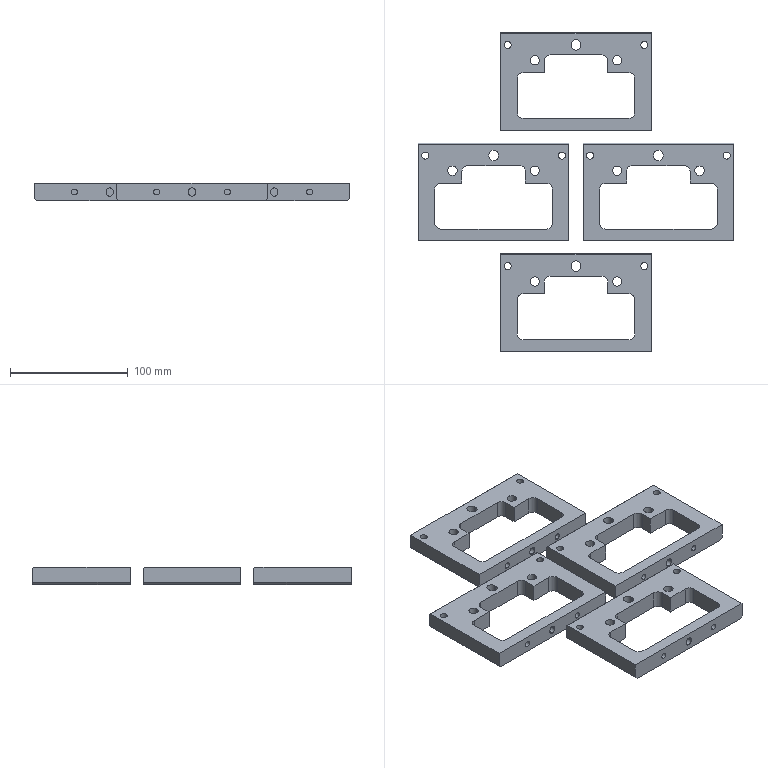NC program | NX | posted with a generic post | part box 268 x 271 x 15 mm
Lines 11494 to 12247 of 34527:
(HOLE_MILLING , TOOL : D4)
N22950 T04 M6
N22952 G54
N22954 G17 G0 G90 X-35. Y112. B0. C0. S9500 M3
N22956 G43 Z30. H4
N22958 Z0.5
N22960 G94 G3 X-34.05 Y111.05 R0.95 F1650.
N22962 X-33.1 Y112. R0.95
N22964 X-33.1 Y112. Z0.1 I-1.9 J0.
N22966 X-33.1 Y112. Z-0.3 I-1.9 J0.
N22968 X-33.1 Y112. Z-0.7 I-1.9 J0.
N22970 X-33.1 Y112. Z-1.1 I-1.9 J0.
N22972 X-33.1 Y112. Z-1.5 I-1.9 J0.
N22974 X-33.1 Y112. Z-1.9 I-1.9 J0.
N22976 X-33.1 Y112. Z-2.3 I-1.9 J0.
N22978 X-33.1 Y112. Z-2.7 I-1.9 J0.
N22980 X-33.1 Y112. Z-3.1 I-1.9 J0.
N22982 X-33.1 Y112. Z-3.5 I-1.9 J0.
N22984 X-33.1 Y112. Z-3.9 I-1.9 J0.
N22986 X-33.1 Y112. Z-4.3 I-1.9 J0.
N22988 X-33.1 Y112. Z-4.7 I-1.9 J0.
N22990 X-33.1 Y112. Z-5.1 I-1.9 J0.
N22992 X-33.1 Y112. Z-5.5 I-1.9 J0.
N22994 X-33.1 Y112. Z-5.9 I-1.9 J0.
N22996 X-33.1 Y112. Z-6.3 I-1.9 J0.
N22998 X-33.1 Y112. Z-6.7 I-1.9 J0.
N23000 X-33.1 Y112. Z-7.1 I-1.9 J0.
N23002 X-33.1 Y112. Z-7.5 I-1.9 J0.
N23004 X-33.1 Y112. Z-7.9 I-1.9 J0.
N23006 X-33.1 Y112. Z-8.3 I-1.9 J0.
N23008 X-33.1 Y112. Z-8.7 I-1.9 J0.
N23010 X-33.1 Y112. Z-9.1 I-1.9 J0.
N23012 X-33.1 Y112. Z-9.5 I-1.9 J0.
N23014 X-33.1 Y112. Z-9.9 I-1.9 J0.
N23016 X-33.1 Y112. Z-10.3 I-1.9 J0.
N23018 X-33.1 Y112. Z-10.7 I-1.9 J0.
N23020 X-33.1 Y112. Z-11.1 I-1.9 J0.
N23022 X-33.1 Y112. Z-11.5 I-1.9 J0.
N23024 X-33.1 Y112. Z-11.9 I-1.9 J0.
N23026 X-33.1 Y112. Z-12.3 I-1.9 J0.
N23028 X-33.1 Y112. Z-12.7 I-1.9 J0.
N23030 X-33.1 Y112. Z-13.1 I-1.9 J0.
N23032 X-33.1 Y112. Z-13.5 I-1.9 J0.
N23034 X-33.1 Y112. Z-13.9 I-1.9 J0.
N23036 X-33.1 Y112. Z-14.3 I-1.9 J0.
N23038 X-33.1 Y112. Z-14.7 I-1.9 J0.
N23040 X-35. Y110.1 Z-15. R-1.9
N23042 X-33.1 Y112. R1.9
N23044 X-35. Y110.1 R-1.9
N23046 X-34.05 Y111.05 R0.95
N23048 X-35. Y112. R0.95
N23050 G0 Z30.
N23052 X35.
N23054 Z0.5
N23056 G3 X35.95 Y111.05 R0.95
N23058 X36.9 Y112. R0.95
N23060 X36.9 Y112. Z0.1 I-1.9 J0.
N23062 X36.9 Y112. Z-0.3 I-1.9 J0.
N23064 X36.9 Y112. Z-0.7 I-1.9 J0.
N23066 X36.9 Y112. Z-1.1 I-1.9 J0.
N23068 X36.9 Y112. Z-1.5 I-1.9 J0.
N23070 X36.9 Y112. Z-1.9 I-1.9 J0.
N23072 X36.9 Y112. Z-2.3 I-1.9 J0.
N23074 X36.9 Y112. Z-2.7 I-1.9 J0.
N23076 X36.9 Y112. Z-3.1 I-1.9 J0.
N23078 X36.9 Y112. Z-3.5 I-1.9 J0.
N23080 X36.9 Y112. Z-3.9 I-1.9 J0.
N23082 X36.9 Y112. Z-4.3 I-1.9 J0.
N23084 X36.9 Y112. Z-4.7 I-1.9 J0.
N23086 X36.9 Y112. Z-5.1 I-1.9 J0.
N23088 X36.9 Y112. Z-5.5 I-1.9 J0.
N23090 X36.9 Y112. Z-5.9 I-1.9 J0.
N23092 X36.9 Y112. Z-6.3 I-1.9 J0.
N23094 X36.9 Y112. Z-6.7 I-1.9 J0.
N23096 X36.9 Y112. Z-7.1 I-1.9 J0.
N23098 X36.9 Y112. Z-7.5 I-1.9 J0.
N23100 X36.9 Y112. Z-7.9 I-1.9 J0.
N23102 X36.9 Y112. Z-8.3 I-1.9 J0.
N23104 X36.9 Y112. Z-8.7 I-1.9 J0.
N23106 X36.9 Y112. Z-9.1 I-1.9 J0.
N23108 X36.9 Y112. Z-9.5 I-1.9 J0.
N23110 X36.9 Y112. Z-9.9 I-1.9 J0.
N23112 X36.9 Y112. Z-10.3 I-1.9 J0.
N23114 X36.9 Y112. Z-10.7 I-1.9 J0.
N23116 X36.9 Y112. Z-11.1 I-1.9 J0.
N23118 X36.9 Y112. Z-11.5 I-1.9 J0.
N23120 X36.9 Y112. Z-11.9 I-1.9 J0.
N23122 X36.9 Y112. Z-12.3 I-1.9 J0.
N23124 X36.9 Y112. Z-12.7 I-1.9 J0.
N23126 X36.9 Y112. Z-13.1 I-1.9 J0.
N23128 X36.9 Y112. Z-13.5 I-1.9 J0.
N23130 X36.9 Y112. Z-13.9 I-1.9 J0.
N23132 X36.9 Y112. Z-14.3 I-1.9 J0.
N23134 X36.9 Y112. Z-14.7 I-1.9 J0.
N23136 X35. Y110.1 Z-15. R-1.9
N23138 X36.9 Y112. R1.9
N23140 X35. Y110.1 R-1.9
N23142 X35.95 Y111.05 R0.95
N23144 X35. Y112. R0.95
N23146 G0 Z30.
N23148 X105. Y18.
N23150 Z0.5
N23152 G3 X105.95 Y17.05 R0.95
N23154 X106.9 Y18. R0.95
N23156 X106.9 Y18. Z0.1 I-1.9 J0.
N23158 X106.9 Y18. Z-0.3 I-1.9 J0.
N23160 X106.9 Y18. Z-0.7 I-1.9 J0.
N23162 X106.9 Y18. Z-1.1 I-1.9 J0.
N23164 X106.9 Y18. Z-1.5 I-1.9 J0.
N23166 X106.9 Y18. Z-1.9 I-1.9 J0.
N23168 X106.9 Y18. Z-2.3 I-1.9 J0.
N23170 X106.9 Y18. Z-2.7 I-1.9 J0.
N23172 X106.9 Y18. Z-3.1 I-1.9 J0.
N23174 X106.9 Y18. Z-3.5 I-1.9 J0.
N23176 X106.9 Y18. Z-3.9 I-1.9 J0.
N23178 X106.9 Y18. Z-4.3 I-1.9 J0.
N23180 X106.9 Y18. Z-4.7 I-1.9 J0.
N23182 X106.9 Y18. Z-5.1 I-1.9 J0.
N23184 X106.9 Y18. Z-5.5 I-1.9 J0.
N23186 X106.9 Y18. Z-5.9 I-1.9 J0.
N23188 X106.9 Y18. Z-6.3 I-1.9 J0.
N23190 X106.9 Y18. Z-6.7 I-1.9 J0.
N23192 X106.9 Y18. Z-7.1 I-1.9 J0.
N23194 X106.9 Y18. Z-7.5 I-1.9 J0.
N23196 X106.9 Y18. Z-7.9 I-1.9 J0.
N23198 X106.9 Y18. Z-8.3 I-1.9 J0.
N23200 X106.9 Y18. Z-8.7 I-1.9 J0.
N23202 X106.9 Y18. Z-9.1 I-1.9 J0.
N23204 X106.9 Y18. Z-9.5 I-1.9 J0.
N23206 X106.9 Y18. Z-9.9 I-1.9 J0.
N23208 X106.9 Y18. Z-10.3 I-1.9 J0.
N23210 X106.9 Y18. Z-10.7 I-1.9 J0.
N23212 X106.9 Y18. Z-11.1 I-1.9 J0.
N23214 X106.9 Y18. Z-11.5 I-1.9 J0.
N23216 X106.9 Y18. Z-11.9 I-1.9 J0.
N23218 X106.9 Y18. Z-12.3 I-1.9 J0.
N23220 X106.9 Y18. Z-12.7 I-1.9 J0.
N23222 X106.9 Y18. Z-13.1 I-1.9 J0.
N23224 X106.9 Y18. Z-13.5 I-1.9 J0.
N23226 X106.9 Y18. Z-13.9 I-1.9 J0.
N23228 X106.9 Y18. Z-14.3 I-1.9 J0.
N23230 X106.9 Y18. Z-14.7 I-1.9 J0.
N23232 X105. Y16.1 Z-15. R-1.9
N23234 X106.9 Y18. R1.9
N23236 X105. Y16.1 R-1.9
N23238 X105.95 Y17.05 R0.95
N23240 X105. Y18. R0.95
N23242 G0 Z30.
N23244 X35.
N23246 Z0.5
N23248 G3 X35.95 Y17.05 R0.95
N23250 X36.9 Y18. R0.95
N23252 X36.9 Y18. Z0.1 I-1.9 J0.
N23254 X36.9 Y18. Z-0.3 I-1.9 J0.
N23256 X36.9 Y18. Z-0.7 I-1.9 J0.
N23258 X36.9 Y18. Z-1.1 I-1.9 J0.
N23260 X36.9 Y18. Z-1.5 I-1.9 J0.
N23262 X36.9 Y18. Z-1.9 I-1.9 J0.
N23264 X36.9 Y18. Z-2.3 I-1.9 J0.
N23266 X36.9 Y18. Z-2.7 I-1.9 J0.
N23268 X36.9 Y18. Z-3.1 I-1.9 J0.
N23270 X36.9 Y18. Z-3.5 I-1.9 J0.
N23272 X36.9 Y18. Z-3.9 I-1.9 J0.
N23274 X36.9 Y18. Z-4.3 I-1.9 J0.
N23276 X36.9 Y18. Z-4.7 I-1.9 J0.
N23278 X36.9 Y18. Z-5.1 I-1.9 J0.
N23280 X36.9 Y18. Z-5.5 I-1.9 J0.
N23282 X36.9 Y18. Z-5.9 I-1.9 J0.
N23284 X36.9 Y18. Z-6.3 I-1.9 J0.
N23286 X36.9 Y18. Z-6.7 I-1.9 J0.
N23288 X36.9 Y18. Z-7.1 I-1.9 J0.
N23290 X36.9 Y18. Z-7.5 I-1.9 J0.
N23292 X36.9 Y18. Z-7.9 I-1.9 J0.
N23294 X36.9 Y18. Z-8.3 I-1.9 J0.
N23296 X36.9 Y18. Z-8.7 I-1.9 J0.
N23298 X36.9 Y18. Z-9.1 I-1.9 J0.
N23300 X36.9 Y18. Z-9.5 I-1.9 J0.
N23302 X36.9 Y18. Z-9.9 I-1.9 J0.
N23304 X36.9 Y18. Z-10.3 I-1.9 J0.
N23306 X36.9 Y18. Z-10.7 I-1.9 J0.
N23308 X36.9 Y18. Z-11.1 I-1.9 J0.
N23310 X36.9 Y18. Z-11.5 I-1.9 J0.
N23312 X36.9 Y18. Z-11.9 I-1.9 J0.
N23314 X36.9 Y18. Z-12.3 I-1.9 J0.
N23316 X36.9 Y18. Z-12.7 I-1.9 J0.
N23318 X36.9 Y18. Z-13.1 I-1.9 J0.
N23320 X36.9 Y18. Z-13.5 I-1.9 J0.
N23322 X36.9 Y18. Z-13.9 I-1.9 J0.
N23324 X36.9 Y18. Z-14.3 I-1.9 J0.
N23326 X36.9 Y18. Z-14.7 I-1.9 J0.
N23328 X35. Y16.1 Z-15. R-1.9
N23330 X36.9 Y18. R1.9
N23332 X35. Y16.1 R-1.9
N23334 X35.95 Y17.05 R0.95
N23336 X35. Y18. R0.95
N23338 G0 Z30.
N23340 Y-76.
N23342 Z0.5
N23344 G3 X35.95 Y-76.95 R0.95
N23346 X36.9 Y-76. R0.95
N23348 X36.9 Y-76. Z0.1 I-1.9 J0.
N23350 X36.9 Y-76. Z-0.3 I-1.9 J0.
N23352 X36.9 Y-76. Z-0.7 I-1.9 J0.
N23354 X36.9 Y-76. Z-1.1 I-1.9 J0.
N23356 X36.9 Y-76. Z-1.5 I-1.9 J0.
N23358 X36.9 Y-76. Z-1.9 I-1.9 J0.
N23360 X36.9 Y-76. Z-2.3 I-1.9 J0.
N23362 X36.9 Y-76. Z-2.7 I-1.9 J0.
N23364 X36.9 Y-76. Z-3.1 I-1.9 J0.
N23366 X36.9 Y-76. Z-3.5 I-1.9 J0.
N23368 X36.9 Y-76. Z-3.9 I-1.9 J0.
N23370 X36.9 Y-76. Z-4.3 I-1.9 J0.
N23372 X36.9 Y-76. Z-4.7 I-1.9 J0.
N23374 X36.9 Y-76. Z-5.1 I-1.9 J0.
N23376 X36.9 Y-76. Z-5.5 I-1.9 J0.
N23378 X36.9 Y-76. Z-5.9 I-1.9 J0.
N23380 X36.9 Y-76. Z-6.3 I-1.9 J0.
N23382 X36.9 Y-76. Z-6.7 I-1.9 J0.
N23384 X36.9 Y-76. Z-7.1 I-1.9 J0.
N23386 X36.9 Y-76. Z-7.5 I-1.9 J0.
N23388 X36.9 Y-76. Z-7.9 I-1.9 J0.
N23390 X36.9 Y-76. Z-8.3 I-1.9 J0.
N23392 X36.9 Y-76. Z-8.7 I-1.9 J0.
N23394 X36.9 Y-76. Z-9.1 I-1.9 J0.
N23396 X36.9 Y-76. Z-9.5 I-1.9 J0.
N23398 X36.9 Y-76. Z-9.9 I-1.9 J0.
N23400 X36.9 Y-76. Z-10.3 I-1.9 J0.
N23402 X36.9 Y-76. Z-10.7 I-1.9 J0.
N23404 X36.9 Y-76. Z-11.1 I-1.9 J0.
N23406 X36.9 Y-76. Z-11.5 I-1.9 J0.
N23408 X36.9 Y-76. Z-11.9 I-1.9 J0.
N23410 X36.9 Y-76. Z-12.3 I-1.9 J0.
N23412 X36.9 Y-76. Z-12.7 I-1.9 J0.
N23414 X36.9 Y-76. Z-13.1 I-1.9 J0.
N23416 X36.9 Y-76. Z-13.5 I-1.9 J0.
N23418 X36.9 Y-76. Z-13.9 I-1.9 J0.
N23420 X36.9 Y-76. Z-14.3 I-1.9 J0.
N23422 X36.9 Y-76. Z-14.7 I-1.9 J0.
N23424 X35. Y-77.9 Z-15. R-1.9
N23426 X36.9 Y-76. R1.9
N23428 X35. Y-77.9 R-1.9
N23430 X35.95 Y-76.95 R0.95
N23432 X35. Y-76. R0.95
N23434 G0 Z30.
N23436 X-35.
N23438 Z0.5
N23440 G3 X-34.05 Y-76.95 R0.95
N23442 X-33.1 Y-76. R0.95
N23444 X-33.1 Y-76. Z0.1 I-1.9 J0.
N23446 X-33.1 Y-76. Z-0.3 I-1.9 J0.
N23448 X-33.1 Y-76. Z-0.7 I-1.9 J0.
N23450 X-33.1 Y-76. Z-1.1 I-1.9 J0.
N23452 X-33.1 Y-76. Z-1.5 I-1.9 J0.
N23454 X-33.1 Y-76. Z-1.9 I-1.9 J0.
N23456 X-33.1 Y-76. Z-2.3 I-1.9 J0.
N23458 X-33.1 Y-76. Z-2.7 I-1.9 J0.
N23460 X-33.1 Y-76. Z-3.1 I-1.9 J0.
N23462 X-33.1 Y-76. Z-3.5 I-1.9 J0.
N23464 X-33.1 Y-76. Z-3.9 I-1.9 J0.
N23466 X-33.1 Y-76. Z-4.3 I-1.9 J0.
N23468 X-33.1 Y-76. Z-4.7 I-1.9 J0.
N23470 X-33.1 Y-76. Z-5.1 I-1.9 J0.
N23472 X-33.1 Y-76. Z-5.5 I-1.9 J0.
N23474 X-33.1 Y-76. Z-5.9 I-1.9 J0.
N23476 X-33.1 Y-76. Z-6.3 I-1.9 J0.
N23478 X-33.1 Y-76. Z-6.7 I-1.9 J0.
N23480 X-33.1 Y-76. Z-7.1 I-1.9 J0.
N23482 X-33.1 Y-76. Z-7.5 I-1.9 J0.
N23484 X-33.1 Y-76. Z-7.9 I-1.9 J0.
N23486 X-33.1 Y-76. Z-8.3 I-1.9 J0.
N23488 X-33.1 Y-76. Z-8.7 I-1.9 J0.
N23490 X-33.1 Y-76. Z-9.1 I-1.9 J0.
N23492 X-33.1 Y-76. Z-9.5 I-1.9 J0.
N23494 X-33.1 Y-76. Z-9.9 I-1.9 J0.
N23496 X-33.1 Y-76. Z-10.3 I-1.9 J0.
N23498 X-33.1 Y-76. Z-10.7 I-1.9 J0.
N23500 X-33.1 Y-76. Z-11.1 I-1.9 J0.
N23502 X-33.1 Y-76. Z-11.5 I-1.9 J0.
N23504 X-33.1 Y-76. Z-11.9 I-1.9 J0.
N23506 X-33.1 Y-76. Z-12.3 I-1.9 J0.
N23508 X-33.1 Y-76. Z-12.7 I-1.9 J0.
N23510 X-33.1 Y-76. Z-13.1 I-1.9 J0.
N23512 X-33.1 Y-76. Z-13.5 I-1.9 J0.
N23514 X-33.1 Y-76. Z-13.9 I-1.9 J0.
N23516 X-33.1 Y-76. Z-14.3 I-1.9 J0.
N23518 X-33.1 Y-76. Z-14.7 I-1.9 J0.
N23520 X-35. Y-77.9 Z-15. R-1.9
N23522 X-33.1 Y-76. R1.9
N23524 X-35. Y-77.9 R-1.9
N23526 X-34.05 Y-76.95 R0.95
N23528 X-35. Y-76. R0.95
N23530 G0 Z30.
N23532 Y18.
N23534 Z0.5
N23536 G3 X-34.05 Y17.05 R0.95
N23538 X-33.1 Y18. R0.95
N23540 X-33.1 Y18. Z0.1 I-1.9 J0.
N23542 X-33.1 Y18. Z-0.3 I-1.9 J0.
N23544 X-33.1 Y18. Z-0.7 I-1.9 J0.
N23546 X-33.1 Y18. Z-1.1 I-1.9 J0.
N23548 X-33.1 Y18. Z-1.5 I-1.9 J0.
N23550 X-33.1 Y18. Z-1.9 I-1.9 J0.
N23552 X-33.1 Y18. Z-2.3 I-1.9 J0.
N23554 X-33.1 Y18. Z-2.7 I-1.9 J0.
N23556 X-33.1 Y18. Z-3.1 I-1.9 J0.
N23558 X-33.1 Y18. Z-3.5 I-1.9 J0.
N23560 X-33.1 Y18. Z-3.9 I-1.9 J0.
N23562 X-33.1 Y18. Z-4.3 I-1.9 J0.
N23564 X-33.1 Y18. Z-4.7 I-1.9 J0.
N23566 X-33.1 Y18. Z-5.1 I-1.9 J0.
N23568 X-33.1 Y18. Z-5.5 I-1.9 J0.
N23570 X-33.1 Y18. Z-5.9 I-1.9 J0.
N23572 X-33.1 Y18. Z-6.3 I-1.9 J0.
N23574 X-33.1 Y18. Z-6.7 I-1.9 J0.
N23576 X-33.1 Y18. Z-7.1 I-1.9 J0.
N23578 X-33.1 Y18. Z-7.5 I-1.9 J0.
N23580 X-33.1 Y18. Z-7.9 I-1.9 J0.
N23582 X-33.1 Y18. Z-8.3 I-1.9 J0.
N23584 X-33.1 Y18. Z-8.7 I-1.9 J0.
N23586 X-33.1 Y18. Z-9.1 I-1.9 J0.
N23588 X-33.1 Y18. Z-9.5 I-1.9 J0.
N23590 X-33.1 Y18. Z-9.9 I-1.9 J0.
N23592 X-33.1 Y18. Z-10.3 I-1.9 J0.
N23594 X-33.1 Y18. Z-10.7 I-1.9 J0.
N23596 X-33.1 Y18. Z-11.1 I-1.9 J0.
N23598 X-33.1 Y18. Z-11.5 I-1.9 J0.
N23600 X-33.1 Y18. Z-11.9 I-1.9 J0.
N23602 X-33.1 Y18. Z-12.3 I-1.9 J0.
N23604 X-33.1 Y18. Z-12.7 I-1.9 J0.
N23606 X-33.1 Y18. Z-13.1 I-1.9 J0.
N23608 X-33.1 Y18. Z-13.5 I-1.9 J0.
N23610 X-33.1 Y18. Z-13.9 I-1.9 J0.
N23612 X-33.1 Y18. Z-14.3 I-1.9 J0.
N23614 X-33.1 Y18. Z-14.7 I-1.9 J0.
N23616 X-35. Y16.1 Z-15. R-1.9
N23618 X-33.1 Y18. R1.9
N23620 X-35. Y16.1 R-1.9
N23622 X-34.05 Y17.05 R0.95
N23624 X-35. Y18. R0.95
N23626 G0 Z30.
N23628 X-105.
N23630 Z0.5
N23632 G3 X-104.05 Y17.05 R0.95
N23634 X-103.1 Y18. R0.95
N23636 X-103.1 Y18. Z0.1 I-1.9 J0.
N23638 X-103.1 Y18. Z-0.3 I-1.9 J0.
N23640 X-103.1 Y18. Z-0.7 I-1.9 J0.
N23642 X-103.1 Y18. Z-1.1 I-1.9 J0.
N23644 X-103.1 Y18. Z-1.5 I-1.9 J0.
N23646 X-103.1 Y18. Z-1.9 I-1.9 J0.
N23648 X-103.1 Y18. Z-2.3 I-1.9 J0.
N23650 X-103.1 Y18. Z-2.7 I-1.9 J0.
N23652 X-103.1 Y18. Z-3.1 I-1.9 J0.
N23654 X-103.1 Y18. Z-3.5 I-1.9 J0.
N23656 X-103.1 Y18. Z-3.9 I-1.9 J0.
N23658 X-103.1 Y18. Z-4.3 I-1.9 J0.
N23660 X-103.1 Y18. Z-4.7 I-1.9 J0.
N23662 X-103.1 Y18. Z-5.1 I-1.9 J0.
N23664 X-103.1 Y18. Z-5.5 I-1.9 J0.
N23666 X-103.1 Y18. Z-5.9 I-1.9 J0.
N23668 X-103.1 Y18. Z-6.3 I-1.9 J0.
N23670 X-103.1 Y18. Z-6.7 I-1.9 J0.
N23672 X-103.1 Y18. Z-7.1 I-1.9 J0.
N23674 X-103.1 Y18. Z-7.5 I-1.9 J0.
N23676 X-103.1 Y18. Z-7.9 I-1.9 J0.
N23678 X-103.1 Y18. Z-8.3 I-1.9 J0.
N23680 X-103.1 Y18. Z-8.7 I-1.9 J0.
N23682 X-103.1 Y18. Z-9.1 I-1.9 J0.
N23684 X-103.1 Y18. Z-9.5 I-1.9 J0.
N23686 X-103.1 Y18. Z-9.9 I-1.9 J0.
N23688 X-103.1 Y18. Z-10.3 I-1.9 J0.
N23690 X-103.1 Y18. Z-10.7 I-1.9 J0.
N23692 X-103.1 Y18. Z-11.1 I-1.9 J0.
N23694 X-103.1 Y18. Z-11.5 I-1.9 J0.
N23696 X-103.1 Y18. Z-11.9 I-1.9 J0.
N23698 X-103.1 Y18. Z-12.3 I-1.9 J0.
N23700 X-103.1 Y18. Z-12.7 I-1.9 J0.
N23702 X-103.1 Y18. Z-13.1 I-1.9 J0.
N23704 X-103.1 Y18. Z-13.5 I-1.9 J0.
N23706 X-103.1 Y18. Z-13.9 I-1.9 J0.
N23708 X-103.1 Y18. Z-14.3 I-1.9 J0.
N23710 X-103.1 Y18. Z-14.7 I-1.9 J0.
N23712 X-105. Y16.1 Z-15. R-1.9
N23714 X-103.1 Y18. R1.9
N23716 X-105. Y16.1 R-1.9
N23718 X-104.05 Y17.05 R0.95
N23720 X-105. Y18. R0.95
N23722 G0 Z30.
(ZLEVEL_PROFILE_COPY , TOOL : D4)
N23724 X-68.65 Y32.83
N23726 Z1.5
N23728 G1 X-68.775 Y32.965 Z1.49 F1000.
N23730 X-69.188 Y33.229 Z1.465
N23732 X-69.557 Y33.358 Z1.444
N23734 X-70.095 Y33.408 Z1.416
N23736 X-70.625 Y33.305 Z1.388
N23738 X-71.105 Y33.058 Z1.359
N23740 X-71.497 Y32.686 Z1.331
N23742 X-71.769 Y32.219 Z1.303
N23744 X-71.9 Y31.695 Z1.274
N23746 Y30.305 Z1.201
N23748 X-71.785 Y29.822 Z1.175
N23750 X-71.61 Y29.473 Z1.155
N23752 X-71.289 Y29.091 Z1.129
N23754 X-70.881 Y28.805 Z1.103
N23756 X-70.412 Y28.635 Z1.077
N23758 X-69.915 Y28.592 Z1.05
N23760 X-69.424 Y28.679 Z1.024
N23762 X-68.973 Y28.89 Z0.998
N23764 X-68.591 Y29.211 Z0.972
N23766 X-68.358 Y29.524 Z0.952
N23768 X-68.187 Y29.9 Z0.93
N23770 X-68.1 Y30.305 Z0.908
N23772 Y31.695 Z0.835
N23774 X-68.212 Y32.172 Z0.81
N23776 X-68.442 Y32.605 Z0.784
N23778 X-68.775 Y32.965 Z0.758
N23780 X-69.188 Y33.229 Z0.733
N23782 X-69.557 Y33.358 Z0.712
N23784 X-70.095 Y33.408 Z0.684
N23786 X-70.625 Y33.305 Z0.656
N23788 X-71.105 Y33.058 Z0.627
N23790 X-71.497 Y32.686 Z0.599
N23792 X-71.769 Y32.219 Z0.571
N23794 X-71.9 Y31.695 Z0.542
N23796 Y30.305 Z0.469
N23798 X-71.785 Y29.822 Z0.443
N23800 X-71.61 Y29.473 Z0.423
N23802 X-71.289 Y29.091 Z0.397
N23804 X-70.881 Y28.805 Z0.371
N23806 X-70.412 Y28.635 Z0.345
N23808 X-69.915 Y28.592 Z0.318
N23810 X-69.424 Y28.679 Z0.292
N23812 X-68.973 Y28.89 Z0.266
N23814 X-68.591 Y29.211 Z0.24
N23816 X-68.358 Y29.524 Z0.22
N23818 X-68.187 Y29.9 Z0.198
N23820 X-68.1 Y30.305 Z0.176
N23822 Y31.695 Z0.103
N23824 X-68.212 Y32.172 Z0.078
N23826 X-68.442 Y32.605 Z0.052
N23828 X-68.775 Y32.965 Z0.026
N23830 X-69.188 Y33.229 Z0.001
N23832 X-69.557 Y33.358 Z-0.02
N23834 X-70.095 Y33.408 Z-0.048
N23836 X-70.625 Y33.305 Z-0.077
N23838 X-71.105 Y33.058 Z-0.105
N23840 X-71.497 Y32.686 Z-0.133
N23842 X-71.769 Y32.219 Z-0.161
N23844 X-71.9 Y31.695 Z-0.19
N23846 Y31.5 Z-0.2
N23848 Y30.5 F1200.
N23850 G3 X-70. Y28.6 R1.9
N23852 X-68.1 Y30.5 R1.9
N23854 G1 Y31.5
N23856 G3 X-70. Y33.4 R1.9
N23858 X-71.9 Y31.5 R1.9
N23860 G1 Y30.652 Z-0.216
N23862 X-71.897 Y30.511 Z-0.219
N23864 X-71.888 Y30.371 Z-0.222
N23866 X-71.877 Y30.23 Z-0.224
N23868 X-71.848 Y30.092 Z-0.227
N23870 X-71.814 Y29.956 Z-0.23
N23872 X-71.768 Y29.823 Z-0.232
N23874 X-71.713 Y29.693 Z-0.235
N23876 X-71.648 Y29.568 Z-0.238
N23878 X-71.574 Y29.449 Z-0.241
N23880 X-71.493 Y29.334 Z-0.243
N23882 X-71.401 Y29.227 Z-0.246
N23884 X-71.304 Y29.125 Z-0.249
N23886 X-71.197 Y29.034 Z-0.251
N23888 X-71.087 Y28.946 Z-0.254
N23890 X-70.966 Y28.873 Z-0.257
N23892 X-70.843 Y28.804 Z-0.259
N23894 X-70.714 Y28.747 Z-0.262
N23896 X-70.582 Y28.699 Z-0.265
N23898 X-70.447 Y28.66 Z-0.268
N23900 X-70.309 Y28.632 Z-0.27
N23902 X-70.17 Y28.614 Z-0.273
N23904 X-70.029 Y28.608 Z-0.276
N23906 X-69.888 Y28.609 Z-0.278
N23908 X-69.748 Y28.625 Z-0.281
N23910 X-69.609 Y28.645 Z-0.284
N23912 X-69.473 Y28.683 Z-0.286
N23914 X-69.339 Y28.724 Z-0.289
N23916 X-69.21 Y28.781 Z-0.292
N23918 X-69.083 Y28.843 Z-0.295
N23920 X-68.963 Y28.916 Z-0.297
N23922 X-68.849 Y28.998 Z-0.3
N23924 X-68.739 Y29.086 Z-0.303
N23926 X-68.634 Y29.18 Z-0.305
N23928 X-68.539 Y29.285 Z-0.308
N23930 X-68.453 Y29.397 Z-0.311
N23932 X-68.375 Y29.515 Z-0.314
N23934 X-68.307 Y29.638 Z-0.316
N23936 X-68.247 Y29.766 Z-0.319
N23938 X-68.198 Y29.898 Z-0.322
N23940 X-68.158 Y30.034 Z-0.324
N23942 X-68.129 Y30.172 Z-0.327
N23944 X-68.116 Y30.313 Z-0.33
N23946 X-68.106 Y30.453 Z-0.332
N23948 X-68.1 Y30.594 Z-0.335
N23950 Y31.442 Z-0.351
N23952 X-68.109 Y31.582 Z-0.354
N23954 X-68.119 Y31.723 Z-0.357
N23956 X-68.142 Y31.862 Z-0.359
N23958 X-68.172 Y32. Z-0.362
N23960 X-68.217 Y32.133 Z-0.365
N23962 X-68.266 Y32.265 Z-0.368
N23964 X-68.33 Y32.39 Z-0.37
N23966 X-68.399 Y32.513 Z-0.373
N23968 X-68.48 Y32.628 Z-0.376
N23970 X-68.568 Y32.738 Z-0.378
N23972 X-68.664 Y32.841 Z-0.381
N23974 X-68.767 Y32.937 Z-0.384
N23976 X-68.877 Y33.025 Z-0.386
N23978 X-68.994 Y33.102 Z-0.389
N23980 X-69.114 Y33.176 Z-0.392
N23982 X-69.243 Y33.234 Z-0.395
N23984 X-69.372 Y33.289 Z-0.397
N23986 X-69.506 Y33.335 Z-0.4
N23988 G3 X-71.9 Y31.5 R1.9
N23990 G1 Y30.652 Z-0.416
N23992 X-71.897 Y30.511 Z-0.419
N23994 X-71.888 Y30.371 Z-0.422
N23996 X-71.877 Y30.23 Z-0.424
N23998 X-71.848 Y30.092 Z-0.427
N24000 X-71.814 Y29.956 Z-0.43
N24002 X-71.768 Y29.823 Z-0.432
N24004 X-71.713 Y29.693 Z-0.435
N24006 X-71.648 Y29.568 Z-0.438
N24008 X-71.574 Y29.449 Z-0.441
N24010 X-71.493 Y29.334 Z-0.443
N24012 X-71.401 Y29.227 Z-0.446
N24014 X-71.304 Y29.125 Z-0.449
N24016 X-71.197 Y29.034 Z-0.451
N24018 X-71.087 Y28.946 Z-0.454
N24020 X-70.966 Y28.873 Z-0.457
N24022 X-70.843 Y28.804 Z-0.459
N24024 X-70.714 Y28.747 Z-0.462
N24026 X-70.582 Y28.699 Z-0.465
N24028 X-70.447 Y28.66 Z-0.468
N24030 X-70.309 Y28.632 Z-0.47
N24032 X-70.17 Y28.614 Z-0.473
N24034 X-70.029 Y28.608 Z-0.476
N24036 X-69.888 Y28.609 Z-0.478
N24038 X-69.748 Y28.625 Z-0.481
N24040 X-69.609 Y28.645 Z-0.484
N24042 X-69.473 Y28.683 Z-0.486
N24044 X-69.339 Y28.724 Z-0.489
N24046 X-69.21 Y28.781 Z-0.492
N24048 X-69.083 Y28.843 Z-0.495
N24050 X-68.963 Y28.916 Z-0.497
N24052 X-68.849 Y28.998 Z-0.5
N24054 X-68.739 Y29.086 Z-0.503
N24056 X-68.634 Y29.18 Z-0.505
N24058 X-68.539 Y29.285 Z-0.508
N24060 X-68.453 Y29.397 Z-0.511
N24062 X-68.375 Y29.515 Z-0.514
N24064 X-68.307 Y29.638 Z-0.516
N24066 X-68.247 Y29.766 Z-0.519
N24068 X-68.198 Y29.898 Z-0.522
N24070 X-68.158 Y30.034 Z-0.524
N24072 X-68.129 Y30.172 Z-0.527
N24074 X-68.116 Y30.313 Z-0.53
N24076 X-68.106 Y30.453 Z-0.532
N24078 X-68.1 Y30.594 Z-0.535
N24080 Y31.442 Z-0.551
N24082 X-68.109 Y31.582 Z-0.554
N24084 X-68.119 Y31.723 Z-0.557
N24086 X-68.142 Y31.862 Z-0.559
N24088 X-68.172 Y32. Z-0.562
N24090 X-68.217 Y32.133 Z-0.565
N24092 X-68.266 Y32.265 Z-0.568
N24094 X-68.33 Y32.39 Z-0.57
N24096 X-68.399 Y32.513 Z-0.573
N24098 X-68.48 Y32.628 Z-0.576
N24100 X-68.568 Y32.738 Z-0.578
N24102 X-68.664 Y32.841 Z-0.581
N24104 X-68.767 Y32.937 Z-0.584
N24106 X-68.877 Y33.025 Z-0.586
N24108 X-68.994 Y33.102 Z-0.589
N24110 X-69.114 Y33.176 Z-0.592
N24112 X-69.243 Y33.234 Z-0.595
N24114 X-69.372 Y33.289 Z-0.597
N24116 X-69.506 Y33.335 Z-0.6
N24118 G3 X-71.9 Y31.5 R1.9
N24120 G1 Y30.652 Z-0.616
N24122 X-71.897 Y30.511 Z-0.619
N24124 X-71.888 Y30.371 Z-0.622
N24126 X-71.877 Y30.23 Z-0.624
N24128 X-71.848 Y30.092 Z-0.627
N24130 X-71.814 Y29.956 Z-0.63
N24132 X-71.768 Y29.823 Z-0.632
N24134 X-71.713 Y29.693 Z-0.635
N24136 X-71.648 Y29.568 Z-0.638
N24138 X-71.574 Y29.449 Z-0.641
N24140 X-71.493 Y29.334 Z-0.643
N24142 X-71.401 Y29.227 Z-0.646
N24144 X-71.304 Y29.125 Z-0.649
N24146 X-71.197 Y29.034 Z-0.651
N24148 X-71.087 Y28.946 Z-0.654
N24150 X-70.966 Y28.873 Z-0.657
N24152 X-70.843 Y28.804 Z-0.659
N24154 X-70.714 Y28.747 Z-0.662
N24156 X-70.582 Y28.699 Z-0.665
N24158 X-70.447 Y28.66 Z-0.668
N24160 X-70.309 Y28.632 Z-0.67
N24162 X-70.17 Y28.614 Z-0.673
N24164 X-70.029 Y28.608 Z-0.676
N24166 X-69.888 Y28.609 Z-0.678
N24168 X-69.748 Y28.625 Z-0.681
N24170 X-69.609 Y28.645 Z-0.684
N24172 X-69.473 Y28.683 Z-0.686
N24174 X-69.339 Y28.724 Z-0.689
N24176 X-69.21 Y28.781 Z-0.692
N24178 X-69.083 Y28.843 Z-0.695
N24180 X-68.963 Y28.916 Z-0.697
N24182 X-68.849 Y28.998 Z-0.7
N24184 X-68.739 Y29.086 Z-0.703
N24186 X-68.634 Y29.18 Z-0.705
N24188 X-68.539 Y29.285 Z-0.708
N24190 X-68.453 Y29.397 Z-0.711
N24192 X-68.375 Y29.515 Z-0.714
N24194 X-68.307 Y29.638 Z-0.716
N24196 X-68.247 Y29.766 Z-0.719
N24198 X-68.198 Y29.898 Z-0.722
N24200 X-68.158 Y30.034 Z-0.724
N24202 X-68.129 Y30.172 Z-0.727
N24204 X-68.116 Y30.313 Z-0.73
N24206 X-68.106 Y30.453 Z-0.732
N24208 X-68.1 Y30.594 Z-0.735
N24210 Y31.442 Z-0.751
N24212 X-68.109 Y31.582 Z-0.754
N24214 X-68.119 Y31.723 Z-0.757
N24216 X-68.142 Y31.862 Z-0.759
N24218 X-68.172 Y32. Z-0.762
N24220 X-68.217 Y32.133 Z-0.765
N24222 X-68.266 Y32.265 Z-0.768
N24224 X-68.33 Y32.39 Z-0.77
N24226 X-68.399 Y32.513 Z-0.773
N24228 X-68.48 Y32.628 Z-0.776
N24230 X-68.568 Y32.738 Z-0.778
N24232 X-68.664 Y32.841 Z-0.781
N24234 X-68.767 Y32.937 Z-0.784
N24236 X-68.877 Y33.025 Z-0.786
N24238 X-68.994 Y33.102 Z-0.789
N24240 X-69.114 Y33.176 Z-0.792
N24242 X-69.243 Y33.234 Z-0.795
N24244 X-69.372 Y33.289 Z-0.797
N24246 X-69.506 Y33.335 Z-0.8
N24248 G3 X-71.9 Y31.5 R1.9
N24250 G1 Y30.652 Z-0.816
N24252 X-71.897 Y30.511 Z-0.819
N24254 X-71.888 Y30.371 Z-0.822
N24256 X-71.877 Y30.23 Z-0.824
N24258 X-71.848 Y30.092 Z-0.827
N24260 X-71.814 Y29.956 Z-0.83
N24262 X-71.768 Y29.823 Z-0.832
N24264 X-71.713 Y29.693 Z-0.835
N24266 X-71.648 Y29.568 Z-0.838
N24268 X-71.574 Y29.449 Z-0.841
N24270 X-71.493 Y29.334 Z-0.843
N24272 X-71.401 Y29.227 Z-0.846
N24274 X-71.304 Y29.125 Z-0.849
N24276 X-71.197 Y29.034 Z-0.851
N24278 X-71.087 Y28.946 Z-0.854
N24280 X-70.966 Y28.873 Z-0.857
N24282 X-70.843 Y28.804 Z-0.859
N24284 X-70.714 Y28.747 Z-0.862
N24286 X-70.582 Y28.699 Z-0.865
N24288 X-70.447 Y28.66 Z-0.868
N24290 X-70.309 Y28.632 Z-0.87
N24292 X-70.17 Y28.614 Z-0.873
N24294 X-70.029 Y28.608 Z-0.876
N24296 X-69.888 Y28.609 Z-0.878
N24298 X-69.748 Y28.625 Z-0.881
N24300 X-69.609 Y28.645 Z-0.884
N24302 X-69.473 Y28.683 Z-0.886
N24304 X-69.339 Y28.724 Z-0.889
N24306 X-69.21 Y28.781 Z-0.892
N24308 X-69.083 Y28.843 Z-0.895
N24310 X-68.963 Y28.916 Z-0.897
N24312 X-68.849 Y28.998 Z-0.9
N24314 X-68.739 Y29.086 Z-0.903
N24316 X-68.634 Y29.18 Z-0.905
N24318 X-68.539 Y29.285 Z-0.908
N24320 X-68.453 Y29.397 Z-0.911
N24322 X-68.375 Y29.515 Z-0.914
N24324 X-68.307 Y29.638 Z-0.916
N24326 X-68.247 Y29.766 Z-0.919
N24328 X-68.198 Y29.898 Z-0.922
N24330 X-68.158 Y30.034 Z-0.924
N24332 X-68.129 Y30.172 Z-0.927
N24334 X-68.116 Y30.313 Z-0.93
N24336 X-68.106 Y30.453 Z-0.932
N24338 X-68.1 Y30.594 Z-0.935
N24340 Y31.442 Z-0.951
N24342 X-68.109 Y31.582 Z-0.954
N24344 X-68.119 Y31.723 Z-0.957
N24346 X-68.142 Y31.862 Z-0.959
N24348 X-68.172 Y32. Z-0.962
N24350 X-68.217 Y32.133 Z-0.965
N24352 X-68.266 Y32.265 Z-0.968
N24354 X-68.33 Y32.39 Z-0.97
N24356 X-68.399 Y32.513 Z-0.973
N24358 X-68.48 Y32.628 Z-0.976
N24360 X-68.568 Y32.738 Z-0.978
N24362 X-68.664 Y32.841 Z-0.981
N24364 X-68.767 Y32.937 Z-0.984
N24366 X-68.877 Y33.025 Z-0.986
N24368 X-68.994 Y33.102 Z-0.989
N24370 X-69.114 Y33.176 Z-0.992
N24372 X-69.243 Y33.234 Z-0.995
N24374 X-69.372 Y33.289 Z-0.997
N24376 X-69.506 Y33.335 Z-1.
N24378 G3 X-71.9 Y31.5 R1.9
N24380 G1 Y30.652 Z-1.016
N24382 X-71.897 Y30.511 Z-1.019
N24384 X-71.888 Y30.371 Z-1.022
N24386 X-71.877 Y30.23 Z-1.024
N24388 X-71.848 Y30.092 Z-1.027
N24390 X-71.814 Y29.956 Z-1.03
N24392 X-71.768 Y29.823 Z-1.032
N24394 X-71.713 Y29.693 Z-1.035
N24396 X-71.648 Y29.568 Z-1.038
N24398 X-71.574 Y29.449 Z-1.041
N24400 X-71.493 Y29.334 Z-1.043
N24402 X-71.401 Y29.227 Z-1.046
N24404 X-71.304 Y29.125 Z-1.049
N24406 X-71.197 Y29.034 Z-1.051
N24408 X-71.087 Y28.946 Z-1.054
N24410 X-70.966 Y28.873 Z-1.057
N24412 X-70.843 Y28.804 Z-1.059
N24414 X-70.714 Y28.747 Z-1.062
N24416 X-70.582 Y28.699 Z-1.065
N24418 X-70.447 Y28.66 Z-1.068
N24420 X-70.309 Y28.632 Z-1.07
N24422 X-70.17 Y28.614 Z-1.073
N24424 X-70.029 Y28.608 Z-1.076
N24426 X-69.888 Y28.609 Z-1.078
N24428 X-69.748 Y28.625 Z-1.081
N24430 X-69.609 Y28.645 Z-1.084
N24432 X-69.473 Y28.683 Z-1.086
N24434 X-69.339 Y28.724 Z-1.089
N24436 X-69.21 Y28.781 Z-1.092
N24438 X-69.083 Y28.843 Z-1.095
N24440 X-68.963 Y28.916 Z-1.097
N24442 X-68.849 Y28.998 Z-1.1
N24444 X-68.739 Y29.086 Z-1.103